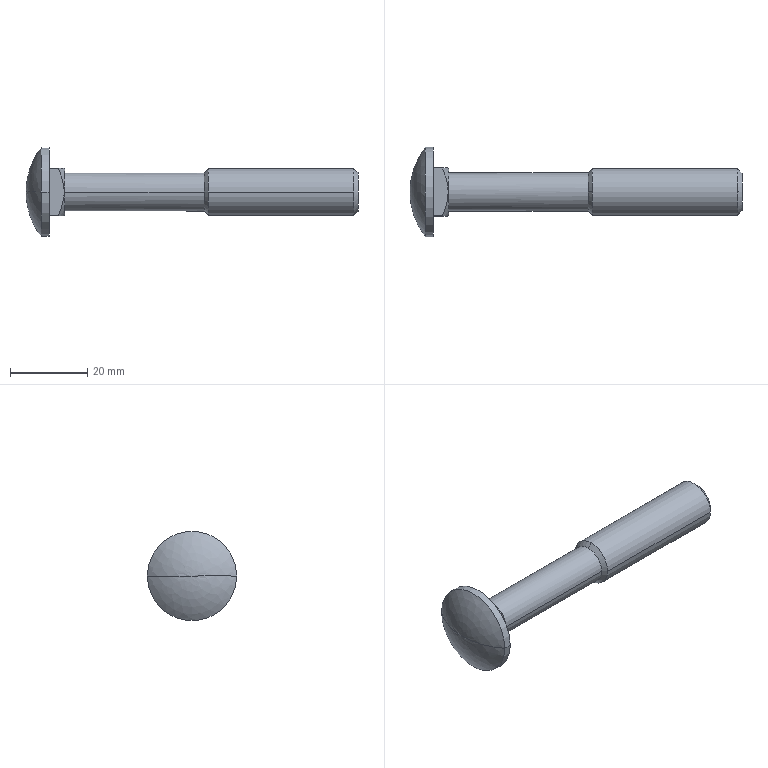Part | SolidWorks | features BaseBody 1 | 1 solid | 21 faces | box 86 x 23.16 x 23.16 mm | volume 9538 mm3 | plane 7 | cylinder 6 | cone 6 | spline 2 | commonest cylinder face diameters 9.853 x2 12 x2 23.16 x2
STEP:
#1=CARTESIAN_POINT('',(-2.,-11.58,0.));
#2=VERTEX_POINT('',#1);
#3=CARTESIAN_POINT('',(-2.,11.58,0.));
#4=VERTEX_POINT('',#3);
#5=CARTESIAN_POINT('',(-2.,0.,0.));
#6=DIRECTION('',(1.,0.,0.));
#7=DIRECTION('',(0.,1.,0.));
#8=AXIS2_PLACEMENT_3D('',#5,#6,#7);
#9=CIRCLE('',#8,11.58);
#10=EDGE_CURVE('',#2,#4,#9,.T.);
#11=ORIENTED_EDGE('',*,*,#10,.F.);
#12=CARTESIAN_POINT('',(-6.,0.,0.));
#13=VERTEX_POINT('',#12);
#14=CARTESIAN_POINT('',(12.762,0.,0.));
#15=DIRECTION('',(0.,0.,-1.));
#16=DIRECTION('',(1.,0.,0.));
#17=AXIS2_PLACEMENT_3D('',#14,#15,#16);
#18=CIRCLE('',#17,18.762);
#19=EDGE_CURVE('',#2,#13,#18,.T.);
#20=ORIENTED_EDGE('',*,*,#19,.T.);
#21=CARTESIAN_POINT('',(12.762,0.,0.));
#22=DIRECTION('',(0.,0.,1.));
#23=DIRECTION('',(1.,0.,0.));
#24=AXIS2_PLACEMENT_3D('',#21,#22,#23);
#25=CIRCLE('',#24,18.762);
#26=EDGE_CURVE('',#4,#13,#25,.T.);
#27=ORIENTED_EDGE('',*,*,#26,.F.);
#28=EDGE_LOOP('',(#11,#20,#27));
#29=FACE_OUTER_BOUND('',#28,.T.);
#30=CARTESIAN_POINT('',(-2.,-11.58,0.));
#31=CARTESIAN_POINT('',(-2.,-11.58,-23.16));
#32=CARTESIAN_POINT('',(-2.,11.58,-23.16));
#33=CARTESIAN_POINT('',(-2.,11.58,0.));
#34=CARTESIAN_POINT('',(-4.616,-8.245,0.));
#35=CARTESIAN_POINT('',(-4.616,-8.245,-16.49));
#36=CARTESIAN_POINT('',(-4.616,8.245,-16.49));
#37=CARTESIAN_POINT('',(-4.616,8.245,0.));
#38=CARTESIAN_POINT('',(-6.,-4.239,0.));
#39=CARTESIAN_POINT('',(-6.,-4.239,-8.477));
#40=CARTESIAN_POINT('',(-6.,4.239,-8.477));
#41=CARTESIAN_POINT('',(-6.,4.239,0.));
#42=CARTESIAN_POINT('',(-6.,0.,0.));
#43=CARTESIAN_POINT('',(-6.,0.,0.));
#44=CARTESIAN_POINT('',(-6.,0.,0.));
#45=CARTESIAN_POINT('',(-6.,0.,0.));
#46=(BOUNDED_SURFACE()B_SPLINE_SURFACE(3,3,((#30,#31,#32,#33),(#34,#35,#36,#37),(#38,#39,#40,#41),(#42,#43,#44,#45)),.UNSPECIFIED.,.F.,.F.,.F.)B_SPLINE_SURFACE_WITH_KNOTS((4,4),(4,4),(0.,1.),(0.,1.),.UNSPECIFIED.)GEOMETRIC_REPRESENTATION_ITEM()RATIONAL_B_SPLINE_SURFACE(((1.,0.3333,0.3333,1.),(0.9635,0.3212,0.3212,0.9635),(0.9635,0.3212,0.3212,0.9635),(1.,0.3333,0.3333,1.)))REPRESENTATION_ITEM('')SURFACE());
#47=ADVANCED_FACE('',(#29),#46,.T.);
#48=CARTESIAN_POINT('',(41.25,0.,6.));
#49=VERTEX_POINT('',#48);
#50=CARTESIAN_POINT('',(41.25,-6.,0.));
#51=VERTEX_POINT('',#50);
#52=CARTESIAN_POINT('',(41.25,0.,0.));
#53=DIRECTION('',(1.,0.,0.));
#54=DIRECTION('',(0.,1.,0.));
#55=AXIS2_PLACEMENT_3D('',#52,#53,#54);
#56=CIRCLE('',#55,6.);
#57=EDGE_CURVE('',#49,#51,#56,.T.);
#58=ORIENTED_EDGE('',*,*,#57,.T.);
#59=CARTESIAN_POINT('',(78.926,-6.,0.));
#60=VERTEX_POINT('',#59);
#61=CARTESIAN_POINT('',(60.625,-6.,0.));
#62=DIRECTION('',(1.,0.,0.));
#63=VECTOR('',#62,1000.);
#64=LINE('',#61,#63);
#65=EDGE_CURVE('',#51,#60,#64,.T.);
#66=ORIENTED_EDGE('',*,*,#65,.T.);
#67=CARTESIAN_POINT('',(78.926,0.,6.));
#68=VERTEX_POINT('',#67);
#69=CARTESIAN_POINT('',(78.926,0.,0.));
#70=DIRECTION('',(-1.,0.,0.));
#71=DIRECTION('',(0.,1.,0.));
#72=AXIS2_PLACEMENT_3D('',#69,#70,#71);
#73=CIRCLE('',#72,6.);
#74=EDGE_CURVE('',#60,#68,#73,.T.);
#75=ORIENTED_EDGE('',*,*,#74,.T.);
#76=CARTESIAN_POINT('',(78.926,6.,0.));
#77=VERTEX_POINT('',#76);
#78=CARTESIAN_POINT('',(78.926,0.,0.));
#79=DIRECTION('',(-1.,0.,0.));
#80=DIRECTION('',(0.,1.,0.));
#81=AXIS2_PLACEMENT_3D('',#78,#79,#80);
#82=CIRCLE('',#81,6.);
#83=EDGE_CURVE('',#68,#77,#82,.T.);
#84=ORIENTED_EDGE('',*,*,#83,.T.);
#85=CARTESIAN_POINT('',(41.25,6.,0.));
#86=VERTEX_POINT('',#85);
#87=CARTESIAN_POINT('',(60.625,6.,0.));
#88=DIRECTION('',(1.,0.,0.));
#89=VECTOR('',#88,1000.);
#90=LINE('',#87,#89);
#91=EDGE_CURVE('',#86,#77,#90,.T.);
#92=ORIENTED_EDGE('',*,*,#91,.F.);
#93=CARTESIAN_POINT('',(41.25,0.,0.));
#94=DIRECTION('',(1.,0.,0.));
#95=DIRECTION('',(0.,1.,0.));
#96=AXIS2_PLACEMENT_3D('',#93,#94,#95);
#97=CIRCLE('',#96,6.);
#98=EDGE_CURVE('',#86,#49,#97,.T.);
#99=ORIENTED_EDGE('',*,*,#98,.T.);
#100=EDGE_LOOP('',(#58,#66,#75,#84,#92,#99));
#101=FACE_OUTER_BOUND('',#100,.T.);
#102=CARTESIAN_POINT('',(60.625,0.,0.));
#103=DIRECTION('',(1.,0.,0.));
#104=DIRECTION('',(0.,1.,0.));
#105=AXIS2_PLACEMENT_3D('',#102,#103,#104);
#106=CYLINDRICAL_SURFACE('',#105,6.);
#107=ADVANCED_FACE('',(#101),#106,.T.);
#108=CARTESIAN_POINT('',(80.,0.,4.926));
#109=VERTEX_POINT('',#108);
#110=CARTESIAN_POINT('',(80.,0.,-4.926));
#111=VERTEX_POINT('',#110);
#112=CARTESIAN_POINT('',(80.,0.,0.));
#113=DIRECTION('',(-1.,0.,0.));
#114=DIRECTION('',(0.,0.,1.));
#115=AXIS2_PLACEMENT_3D('',#112,#113,#114);
#116=CIRCLE('',#115,4.926);
#117=EDGE_CURVE('',#109,#111,#116,.T.);
#118=ORIENTED_EDGE('',*,*,#117,.T.);
#119=CARTESIAN_POINT('',(78.926,0.,-6.));
#120=VERTEX_POINT('',#119);
#121=CARTESIAN_POINT('',(78.926,0.,-6.));
#122=DIRECTION('',(-0.7071,0.,-0.7071));
#123=VECTOR('',#122,1000.);
#124=LINE('',#121,#123);
#125=EDGE_CURVE('',#111,#120,#124,.T.);
#126=ORIENTED_EDGE('',*,*,#125,.T.);
#127=CARTESIAN_POINT('',(78.926,0.,0.));
#128=DIRECTION('',(-1.,0.,0.));
#129=DIRECTION('',(0.,1.,0.));
#130=AXIS2_PLACEMENT_3D('',#127,#128,#129);
#131=CIRCLE('',#130,6.);
#132=EDGE_CURVE('',#77,#120,#131,.T.);
#133=ORIENTED_EDGE('',*,*,#132,.F.);
#134=ORIENTED_EDGE('',*,*,#83,.F.);
#135=CARTESIAN_POINT('',(78.926,0.,6.));
#136=DIRECTION('',(-0.7071,0.,0.7071));
#137=VECTOR('',#136,1000.);
#138=LINE('',#135,#137);
#139=EDGE_CURVE('',#109,#68,#138,.T.);
#140=ORIENTED_EDGE('',*,*,#139,.F.);
#141=EDGE_LOOP('',(#118,#126,#133,#134,#140));
#142=FACE_OUTER_BOUND('',#141,.T.);
#143=CARTESIAN_POINT('',(78.926,0.,0.));
#144=DIRECTION('',(-1.,0.,0.));
#145=DIRECTION('',(0.,0.,1.));
#146=AXIS2_PLACEMENT_3D('',#143,#144,#145);
#147=CONICAL_SURFACE('',#146,6.,0.7854);
#148=ADVANCED_FACE('',(#142),#147,.T.);
#149=CARTESIAN_POINT('',(40.176,4.926,0.));
#150=VERTEX_POINT('',#149);
#151=CARTESIAN_POINT('',(40.176,0.,4.926));
#152=VERTEX_POINT('',#151);
#153=CARTESIAN_POINT('',(40.176,0.,0.));
#154=DIRECTION('',(1.,0.,0.));
#155=DIRECTION('',(0.,1.,0.));
#156=AXIS2_PLACEMENT_3D('',#153,#154,#155);
#157=CIRCLE('',#156,4.926);
#158=EDGE_CURVE('',#150,#152,#157,.T.);
#159=ORIENTED_EDGE('',*,*,#158,.T.);
#160=CARTESIAN_POINT('',(41.25,0.,6.));
#161=DIRECTION('',(0.7071,0.,0.7071));
#162=VECTOR('',#161,1000.);
#163=LINE('',#160,#162);
#164=EDGE_CURVE('',#152,#49,#163,.T.);
#165=ORIENTED_EDGE('',*,*,#164,.T.);
#166=ORIENTED_EDGE('',*,*,#98,.F.);
#167=CARTESIAN_POINT('',(41.25,0.,-6.));
#168=VERTEX_POINT('',#167);
#169=CARTESIAN_POINT('',(41.25,0.,0.));
#170=DIRECTION('',(1.,0.,0.));
#171=DIRECTION('',(0.,1.,0.));
#172=AXIS2_PLACEMENT_3D('',#169,#170,#171);
#173=CIRCLE('',#172,6.);
#174=EDGE_CURVE('',#168,#86,#173,.T.);
#175=ORIENTED_EDGE('',*,*,#174,.F.);
#176=CARTESIAN_POINT('',(40.176,0.,-4.926));
#177=VERTEX_POINT('',#176);
#178=CARTESIAN_POINT('',(41.25,0.,-6.));
#179=DIRECTION('',(0.7071,0.,-0.7071));
#180=VECTOR('',#179,1000.);
#181=LINE('',#178,#180);
#182=EDGE_CURVE('',#177,#168,#181,.T.);
#183=ORIENTED_EDGE('',*,*,#182,.F.);
#184=CARTESIAN_POINT('',(40.176,0.,0.));
#185=DIRECTION('',(1.,0.,0.));
#186=DIRECTION('',(0.,1.,0.));
#187=AXIS2_PLACEMENT_3D('',#184,#185,#186);
#188=CIRCLE('',#187,4.926);
#189=EDGE_CURVE('',#177,#150,#188,.T.);
#190=ORIENTED_EDGE('',*,*,#189,.T.);
#191=EDGE_LOOP('',(#159,#165,#166,#175,#183,#190));
#192=FACE_OUTER_BOUND('',#191,.T.);
#193=CARTESIAN_POINT('',(41.25,0.,0.));
#194=DIRECTION('',(1.,0.,0.));
#195=DIRECTION('',(0.,0.,-1.));
#196=AXIS2_PLACEMENT_3D('',#193,#194,#195);
#197=CONICAL_SURFACE('',#196,6.,0.7854);
#198=ADVANCED_FACE('',(#192),#197,.T.);
#199=CARTESIAN_POINT('',(4.,4.926,0.));
#200=VERTEX_POINT('',#199);
#201=CARTESIAN_POINT('',(4.,-4.926,0.));
#202=VERTEX_POINT('',#201);
#203=CARTESIAN_POINT('',(4.,0.,0.));
#204=DIRECTION('',(1.,0.,0.));
#205=DIRECTION('',(0.,1.,0.));
#206=AXIS2_PLACEMENT_3D('',#203,#204,#205);
#207=CIRCLE('',#206,4.926);
#208=EDGE_CURVE('',#200,#202,#207,.T.);
#209=ORIENTED_EDGE('',*,*,#208,.T.);
#210=CARTESIAN_POINT('',(40.176,-4.926,0.));
#211=VERTEX_POINT('',#210);
#212=CARTESIAN_POINT('',(22.088,-4.926,0.));
#213=DIRECTION('',(1.,0.,0.));
#214=VECTOR('',#213,1000.);
#215=LINE('',#212,#214);
#216=EDGE_CURVE('',#202,#211,#215,.T.);
#217=ORIENTED_EDGE('',*,*,#216,.T.);
#218=CARTESIAN_POINT('',(40.176,0.,0.));
#219=DIRECTION('',(1.,0.,0.));
#220=DIRECTION('',(0.,1.,0.));
#221=AXIS2_PLACEMENT_3D('',#218,#219,#220);
#222=CIRCLE('',#221,4.926);
#223=EDGE_CURVE('',#152,#211,#222,.T.);
#224=ORIENTED_EDGE('',*,*,#223,.F.);
#225=ORIENTED_EDGE('',*,*,#158,.F.);
#226=CARTESIAN_POINT('',(22.088,4.926,0.));
#227=DIRECTION('',(1.,0.,0.));
#228=VECTOR('',#227,1000.);
#229=LINE('',#226,#228);
#230=EDGE_CURVE('',#200,#150,#229,.T.);
#231=ORIENTED_EDGE('',*,*,#230,.F.);
#232=EDGE_LOOP('',(#209,#217,#224,#225,#231));
#233=FACE_OUTER_BOUND('',#232,.T.);
#234=CARTESIAN_POINT('',(22.088,0.,0.));
#235=DIRECTION('',(1.,0.,0.));
#236=DIRECTION('',(0.,1.,0.));
#237=AXIS2_PLACEMENT_3D('',#234,#235,#236);
#238=CYLINDRICAL_SURFACE('',#237,4.926);
#239=ADVANCED_FACE('',(#233),#238,.T.);
#240=CARTESIAN_POINT('',(4.,0.,-6.));
#241=VERTEX_POINT('',#240);
#242=CARTESIAN_POINT('',(4.,0.,6.));
#243=VERTEX_POINT('',#242);
#244=CARTESIAN_POINT('',(4.,0.,0.));
#245=DIRECTION('',(1.,0.,0.));
#246=DIRECTION('',(0.,0.,1.));
#247=AXIS2_PLACEMENT_3D('',#244,#245,#246);
#248=CIRCLE('',#247,6.);
#249=EDGE_CURVE('',#241,#243,#248,.T.);
#250=ORIENTED_EDGE('',*,*,#249,.F.);
#251=CARTESIAN_POINT('',(3.876,0.,-6.215));
#252=VERTEX_POINT('',#251);
#253=CARTESIAN_POINT('',(2.38,0.,-8.806));
#254=DIRECTION('',(-0.5,0.,-0.866));
#255=VECTOR('',#254,1000.);
#256=LINE('',#253,#255);
#257=EDGE_CURVE('',#241,#252,#256,.T.);
#258=ORIENTED_EDGE('',*,*,#257,.T.);
#259=CARTESIAN_POINT('',(2.39,6.215,-6.215));
#260=VERTEX_POINT('',#259);
#261=CARTESIAN_POINT('',(3.876,0.,-6.215));
#262=CARTESIAN_POINT('',(3.876,1.07,-6.215));
#263=CARTESIAN_POINT('',(3.711,2.121,-6.215));
#264=CARTESIAN_POINT('',(3.302,3.681,-6.215));
#265=CARTESIAN_POINT('',(3.141,4.197,-6.215));
#266=CARTESIAN_POINT('',(2.786,5.213,-6.215));
#267=CARTESIAN_POINT('',(2.593,5.716,-6.215));
#268=CARTESIAN_POINT('',(2.39,6.215,-6.215));
#269=B_SPLINE_CURVE_WITH_KNOTS('',3,(#261,#262,#263,#264,#265,#266,#267,#268),.UNSPECIFIED.,.F.,.F.,(4,2,2,4),(0.006403,0.009604,0.0112,0.01281),.UNSPECIFIED.);
#270=EDGE_CURVE('',#252,#260,#269,.T.);
#271=ORIENTED_EDGE('',*,*,#270,.T.);
#272=CARTESIAN_POINT('',(2.39,6.215,6.215));
#273=VERTEX_POINT('',#272);
#274=CARTESIAN_POINT('',(2.39,6.215,-6.215));
#275=CARTESIAN_POINT('',(2.796,6.215,-5.22));
#276=CARTESIAN_POINT('',(3.161,6.215,-4.214));
#277=CARTESIAN_POINT('',(3.569,6.215,-2.666));
#278=CARTESIAN_POINT('',(3.68,6.215,-2.143));
#279=CARTESIAN_POINT('',(3.834,6.215,-1.079));
#280=CARTESIAN_POINT('',(3.876,6.215,-0.535));
#281=CARTESIAN_POINT('',(3.876,6.215,1.07));
#282=CARTESIAN_POINT('',(3.711,6.215,2.121));
#283=CARTESIAN_POINT('',(3.302,6.215,3.681));
#284=CARTESIAN_POINT('',(3.141,6.215,4.197));
#285=CARTESIAN_POINT('',(2.786,6.215,5.213));
#286=CARTESIAN_POINT('',(2.593,6.215,5.716));
#287=CARTESIAN_POINT('',(2.39,6.215,6.215));
#288=B_SPLINE_CURVE_WITH_KNOTS('',3,(#274,#275,#276,#277,#278,#279,#280,#281,#282,#283,#284,#285,#286,#287),.UNSPECIFIED.,.F.,.F.,(4,2,2,2,2,2,4),(0.,0.003201,0.004802,0.006403,0.009604,0.0112,0.01281),.UNSPECIFIED.);
#289=EDGE_CURVE('',#260,#273,#288,.T.);
#290=ORIENTED_EDGE('',*,*,#289,.T.);
#291=CARTESIAN_POINT('',(3.876,0.,6.215));
#292=VERTEX_POINT('',#291);
#293=CARTESIAN_POINT('',(2.39,6.215,6.215));
#294=CARTESIAN_POINT('',(2.796,5.22,6.215));
#295=CARTESIAN_POINT('',(3.161,4.214,6.215));
#296=CARTESIAN_POINT('',(3.569,2.666,6.215));
#297=CARTESIAN_POINT('',(3.68,2.143,6.215));
#298=CARTESIAN_POINT('',(3.834,1.079,6.215));
#299=CARTESIAN_POINT('',(3.876,0.5349,6.215));
#300=CARTESIAN_POINT('',(3.876,0.,6.215));
#301=B_SPLINE_CURVE_WITH_KNOTS('',3,(#293,#294,#295,#296,#297,#298,#299,#300),.UNSPECIFIED.,.F.,.F.,(4,2,2,4),(0.,0.003201,0.004802,0.006403),.UNSPECIFIED.);
#302=EDGE_CURVE('',#273,#292,#301,.T.);
#303=ORIENTED_EDGE('',*,*,#302,.T.);
#304=CARTESIAN_POINT('',(2.38,0.,8.806));
#305=DIRECTION('',(-0.5,0.,0.866));
#306=VECTOR('',#305,1000.);
#307=LINE('',#304,#306);
#308=EDGE_CURVE('',#243,#292,#307,.T.);
#309=ORIENTED_EDGE('',*,*,#308,.F.);
#310=EDGE_LOOP('',(#250,#258,#271,#290,#303,#309));
#311=FACE_OUTER_BOUND('',#310,.T.);
#312=CARTESIAN_POINT('',(2.38,0.,0.));
#313=DIRECTION('',(-1.,0.,0.));
#314=DIRECTION('',(0.,0.,1.));
#315=AXIS2_PLACEMENT_3D('',#312,#313,#314);
#316=CONICAL_SURFACE('',#315,8.806,1.047);
#317=ADVANCED_FACE('',(#311),#316,.T.);
#318=CARTESIAN_POINT('',(-2.,0.,0.));
#319=DIRECTION('',(1.,0.,0.));
#320=DIRECTION('',(0.,1.,0.));
#321=AXIS2_PLACEMENT_3D('',#318,#319,#320);
#322=CIRCLE('',#321,11.58);
#323=EDGE_CURVE('',#4,#2,#322,.T.);
#324=ORIENTED_EDGE('',*,*,#323,.T.);
#325=CARTESIAN_POINT('',(0.,-11.58,0.));
#326=VERTEX_POINT('',#325);
#327=CARTESIAN_POINT('',(-1.,-11.58,0.));
#328=DIRECTION('',(1.,0.,0.));
#329=VECTOR('',#328,1000.);
#330=LINE('',#327,#329);
#331=EDGE_CURVE('',#2,#326,#330,.T.);
#332=ORIENTED_EDGE('',*,*,#331,.T.);
#333=CARTESIAN_POINT('',(0.,11.58,0.));
#334=VERTEX_POINT('',#333);
#335=CARTESIAN_POINT('',(0.,0.,0.));
#336=DIRECTION('',(1.,0.,0.));
#337=DIRECTION('',(0.,1.,0.));
#338=AXIS2_PLACEMENT_3D('',#335,#336,#337);
#339=CIRCLE('',#338,11.58);
#340=EDGE_CURVE('',#334,#326,#339,.T.);
#341=ORIENTED_EDGE('',*,*,#340,.F.);
#342=CARTESIAN_POINT('',(-1.,11.58,0.));
#343=DIRECTION('',(1.,0.,0.));
#344=VECTOR('',#343,1000.);
#345=LINE('',#342,#344);
#346=EDGE_CURVE('',#4,#334,#345,.T.);
#347=ORIENTED_EDGE('',*,*,#346,.F.);
#348=EDGE_LOOP('',(#324,#332,#341,#347));
#349=FACE_OUTER_BOUND('',#348,.T.);
#350=CARTESIAN_POINT('',(-1.,0.,0.));
#351=DIRECTION('',(1.,0.,0.));
#352=DIRECTION('',(0.,1.,0.));
#353=AXIS2_PLACEMENT_3D('',#350,#351,#352);
#354=CYLINDRICAL_SURFACE('',#353,11.58);
#355=ADVANCED_FACE('',(#349),#354,.T.);
#356=ORIENTED_EDGE('',*,*,#65,.F.);
#357=CARTESIAN_POINT('',(41.25,0.,0.));
#358=DIRECTION('',(1.,0.,0.));
#359=DIRECTION('',(0.,1.,0.));
#360=AXIS2_PLACEMENT_3D('',#357,#358,#359);
#361=CIRCLE('',#360,6.);
#362=EDGE_CURVE('',#51,#168,#361,.T.);
#363=ORIENTED_EDGE('',*,*,#362,.T.);
#364=ORIENTED_EDGE('',*,*,#174,.T.);
#365=ORIENTED_EDGE('',*,*,#91,.T.);
#366=ORIENTED_EDGE('',*,*,#132,.T.);
#367=CARTESIAN_POINT('',(78.926,0.,0.));
#368=DIRECTION('',(-1.,0.,0.));
#369=DIRECTION('',(0.,1.,0.));
#370=AXIS2_PLACEMENT_3D('',#367,#368,#369);
#371=CIRCLE('',#370,6.);
#372=EDGE_CURVE('',#120,#60,#371,.T.);
#373=ORIENTED_EDGE('',*,*,#372,.T.);
#374=EDGE_LOOP('',(#356,#363,#364,#365,#366,#373));
#375=FACE_OUTER_BOUND('',#374,.T.);
#376=CARTESIAN_POINT('',(60.625,0.,0.));
#377=DIRECTION('',(1.,0.,0.));
#378=DIRECTION('',(0.,1.,0.));
#379=AXIS2_PLACEMENT_3D('',#376,#377,#378);
#380=CYLINDRICAL_SURFACE('',#379,6.);
#381=ADVANCED_FACE('',(#375),#380,.T.);
#382=ORIENTED_EDGE('',*,*,#125,.F.);
#383=CARTESIAN_POINT('',(80.,0.,0.));
#384=DIRECTION('',(-1.,0.,0.));
#385=DIRECTION('',(0.,0.,1.));
#386=AXIS2_PLACEMENT_3D('',#383,#384,#385);
#387=CIRCLE('',#386,4.926);
#388=EDGE_CURVE('',#111,#109,#387,.T.);
#389=ORIENTED_EDGE('',*,*,#388,.T.);
#390=ORIENTED_EDGE('',*,*,#139,.T.);
#391=ORIENTED_EDGE('',*,*,#74,.F.);
#392=ORIENTED_EDGE('',*,*,#372,.F.);
#393=EDGE_LOOP('',(#382,#389,#390,#391,#392));
#394=FACE_OUTER_BOUND('',#393,.T.);
#395=CARTESIAN_POINT('',(78.926,0.,0.));
#396=DIRECTION('',(-1.,0.,0.));
#397=DIRECTION('',(0.,0.,1.));
#398=AXIS2_PLACEMENT_3D('',#395,#396,#397);
#399=CONICAL_SURFACE('',#398,6.,0.7854);
#400=ADVANCED_FACE('',(#394),#399,.T.);
#401=ORIENTED_EDGE('',*,*,#164,.F.);
#402=ORIENTED_EDGE('',*,*,#223,.T.);
#403=CARTESIAN_POINT('',(40.176,0.,0.));
#404=DIRECTION('',(1.,0.,0.));
#405=DIRECTION('',(0.,1.,0.));
#406=AXIS2_PLACEMENT_3D('',#403,#404,#405);
#407=CIRCLE('',#406,4.926);
#408=EDGE_CURVE('',#211,#177,#407,.T.);
#409=ORIENTED_EDGE('',*,*,#408,.T.);
#410=ORIENTED_EDGE('',*,*,#182,.T.);
#411=ORIENTED_EDGE('',*,*,#362,.F.);
#412=ORIENTED_EDGE('',*,*,#57,.F.);
#413=EDGE_LOOP('',(#401,#402,#409,#410,#411,#412));
#414=FACE_OUTER_BOUND('',#413,.T.);
#415=CARTESIAN_POINT('',(41.25,0.,0.));
#416=DIRECTION('',(1.,0.,0.));
#417=DIRECTION('',(0.,0.,-1.));
#418=AXIS2_PLACEMENT_3D('',#415,#416,#417);
#419=CONICAL_SURFACE('',#418,6.,0.7854);
#420=ADVANCED_FACE('',(#414),#419,.T.);
#421=ORIENTED_EDGE('',*,*,#117,.F.);
#422=ORIENTED_EDGE('',*,*,#388,.F.);
#423=EDGE_LOOP('',(#421,#422));
#424=FACE_OUTER_BOUND('',#423,.T.);
#425=CARTESIAN_POINT('',(80.,3.,0.));
#426=DIRECTION('',(1.,0.,0.));
#427=DIRECTION('',(0.,1.,0.));
#428=AXIS2_PLACEMENT_3D('',#425,#426,#427);
#429=PLANE('',#428);
#430=ADVANCED_FACE('',(#424),#429,.T.);
#431=ORIENTED_EDGE('',*,*,#216,.F.);
#432=CARTESIAN_POINT('',(4.,0.,0.));
#433=DIRECTION('',(1.,0.,0.));
#434=DIRECTION('',(0.,1.,0.));
#435=AXIS2_PLACEMENT_3D('',#432,#433,#434);
#436=CIRCLE('',#435,4.926);
#437=EDGE_CURVE('',#202,#200,#436,.T.);
#438=ORIENTED_EDGE('',*,*,#437,.T.);
#439=ORIENTED_EDGE('',*,*,#230,.T.);
#440=ORIENTED_EDGE('',*,*,#189,.F.);
#441=ORIENTED_EDGE('',*,*,#408,.F.);
#442=EDGE_LOOP('',(#431,#438,#439,#440,#441));
#443=FACE_OUTER_BOUND('',#442,.T.);
#444=CARTESIAN_POINT('',(22.088,0.,0.));
#445=DIRECTION('',(1.,0.,0.));
#446=DIRECTION('',(0.,1.,0.));
#447=AXIS2_PLACEMENT_3D('',#444,#445,#446);
#448=CYLINDRICAL_SURFACE('',#447,4.926);
#449=ADVANCED_FACE('',(#443),#448,.T.);
#450=ORIENTED_EDGE('',*,*,#208,.F.);
#451=ORIENTED_EDGE('',*,*,#437,.F.);
#452=EDGE_LOOP('',(#450,#451));
#453=FACE_BOUND('',#452,.T.);
#454=CARTESIAN_POINT('',(4.,0.,0.));
#455=DIRECTION('',(1.,0.,0.));
#456=DIRECTION('',(0.,0.,1.));
#457=AXIS2_PLACEMENT_3D('',#454,#455,#456);
#458=CIRCLE('',#457,6.);
#459=EDGE_CURVE('',#243,#241,#458,.T.);
#460=ORIENTED_EDGE('',*,*,#459,.T.);
#461=ORIENTED_EDGE('',*,*,#249,.T.);
#462=EDGE_LOOP('',(#460,#461));
#463=FACE_OUTER_BOUND('',#462,.T.);
#464=CARTESIAN_POINT('',(4.,0.,0.));
#465=DIRECTION('',(1.,0.,0.));
#466=DIRECTION('',(0.,0.,-1.));
#467=AXIS2_PLACEMENT_3D('',#464,#465,#466);
#468=PLANE('',#467);
#469=ADVANCED_FACE('',(#453,#463),#468,.T.);
#470=ORIENTED_EDGE('',*,*,#257,.F.);
#471=ORIENTED_EDGE('',*,*,#459,.F.);
#472=ORIENTED_EDGE('',*,*,#308,.T.);
#473=CARTESIAN_POINT('',(2.39,-6.215,6.215));
#474=VERTEX_POINT('',#473);
#475=CARTESIAN_POINT('',(3.876,0.,6.215));
#476=CARTESIAN_POINT('',(3.876,-1.07,6.215));
#477=CARTESIAN_POINT('',(3.711,-2.121,6.215));
#478=CARTESIAN_POINT('',(3.302,-3.681,6.215));
#479=CARTESIAN_POINT('',(3.141,-4.197,6.215));
#480=CARTESIAN_POINT('',(2.786,-5.213,6.215));
#481=CARTESIAN_POINT('',(2.593,-5.716,6.215));
#482=CARTESIAN_POINT('',(2.39,-6.215,6.215));
#483=B_SPLINE_CURVE_WITH_KNOTS('',3,(#475,#476,#477,#478,#479,#480,#481,#482),.UNSPECIFIED.,.F.,.F.,(4,2,2,4),(0.006403,0.009604,0.0112,0.01281),.UNSPECIFIED.);
#484=EDGE_CURVE('',#292,#474,#483,.T.);
#485=ORIENTED_EDGE('',*,*,#484,.T.);
#486=CARTESIAN_POINT('',(2.39,-6.215,-6.215));
#487=VERTEX_POINT('',#486);
#488=CARTESIAN_POINT('',(2.39,-6.215,6.215));
#489=CARTESIAN_POINT('',(2.796,-6.215,5.22));
#490=CARTESIAN_POINT('',(3.161,-6.215,4.214));
#491=CARTESIAN_POINT('',(3.569,-6.215,2.666));
#492=CARTESIAN_POINT('',(3.68,-6.215,2.143));
#493=CARTESIAN_POINT('',(3.834,-6.215,1.079));
#494=CARTESIAN_POINT('',(3.876,-6.215,0.535));
#495=CARTESIAN_POINT('',(3.876,-6.215,-1.07));
#496=CARTESIAN_POINT('',(3.711,-6.215,-2.121));
#497=CARTESIAN_POINT('',(3.302,-6.215,-3.681));
#498=CARTESIAN_POINT('',(3.141,-6.215,-4.197));
#499=CARTESIAN_POINT('',(2.786,-6.215,-5.213));
#500=CARTESIAN_POINT('',(2.593,-6.215,-5.716));
#501=CARTESIAN_POINT('',(2.39,-6.215,-6.215));
#502=B_SPLINE_CURVE_WITH_KNOTS('',3,(#488,#489,#490,#491,#492,#493,#494,#495,#496,#497,#498,#499,#500,#501),.UNSPECIFIED.,.F.,.F.,(4,2,2,2,2,2,4),(0.,0.003201,0.004802,0.006403,0.009604,0.0112,0.01281),.UNSPECIFIED.);
#503=EDGE_CURVE('',#474,#487,#502,.T.);
#504=ORIENTED_EDGE('',*,*,#503,.T.);
#505=CARTESIAN_POINT('',(2.39,-6.215,-6.215));
#506=CARTESIAN_POINT('',(2.796,-5.22,-6.215));
#507=CARTESIAN_POINT('',(3.161,-4.214,-6.215));
#508=CARTESIAN_POINT('',(3.569,-2.666,-6.215));
#509=CARTESIAN_POINT('',(3.68,-2.143,-6.215));
#510=CARTESIAN_POINT('',(3.834,-1.079,-6.215));
#511=CARTESIAN_POINT('',(3.876,-0.5349,-6.215));
#512=CARTESIAN_POINT('',(3.876,0.,-6.215));
#513=B_SPLINE_CURVE_WITH_KNOTS('',3,(#505,#506,#507,#508,#509,#510,#511,#512),.UNSPECIFIED.,.F.,.F.,(4,2,2,4),(0.,0.003201,0.004802,0.006403),.UNSPECIFIED.);
#514=EDGE_CURVE('',#487,#252,#513,.T.);
#515=ORIENTED_EDGE('',*,*,#514,.T.);
#516=EDGE_LOOP('',(#470,#471,#472,#485,#504,#515));
#517=FACE_OUTER_BOUND('',#516,.T.);
#518=CARTESIAN_POINT('',(2.38,0.,0.));
#519=DIRECTION('',(-1.,0.,0.));
#520=DIRECTION('',(0.,0.,1.));
#521=AXIS2_PLACEMENT_3D('',#518,#519,#520);
#522=CONICAL_SURFACE('',#521,8.806,1.047);
#523=ADVANCED_FACE('',(#517),#522,.T.);
#524=CARTESIAN_POINT('',(0.,6.215,-6.215));
#525=VERTEX_POINT('',#524);
#526=CARTESIAN_POINT('',(0.,6.215,6.215));
#527=VERTEX_POINT('',#526);
#528=CARTESIAN_POINT('',(0.,6.215,0.));
#529=DIRECTION('',(0.,0.,1.));
#530=VECTOR('',#529,1000.);
#531=LINE('',#528,#530);
#532=EDGE_CURVE('',#525,#527,#531,.T.);
#533=ORIENTED_EDGE('',*,*,#532,.T.);
#534=CARTESIAN_POINT('',(0.,6.215,6.215));
#535=DIRECTION('',(1.,0.,0.));
#536=VECTOR('',#535,1000.);
#537=LINE('',#534,#536);
#538=EDGE_CURVE('',#527,#273,#537,.T.);
#539=ORIENTED_EDGE('',*,*,#538,.T.);
#540=ORIENTED_EDGE('',*,*,#289,.F.);
#541=CARTESIAN_POINT('',(0.,6.215,-6.215));
#542=DIRECTION('',(-1.,0.,0.));
#543=VECTOR('',#542,1000.);
#544=LINE('',#541,#543);
#545=EDGE_CURVE('',#260,#525,#544,.T.);
#546=ORIENTED_EDGE('',*,*,#545,.T.);
#547=EDGE_LOOP('',(#533,#539,#540,#546));
#548=FACE_OUTER_BOUND('',#547,.T.);
#549=CARTESIAN_POINT('',(0.,6.215,0.));
#550=DIRECTION('',(0.,1.,0.));
#551=DIRECTION('',(0.,0.,1.));
#552=AXIS2_PLACEMENT_3D('',#549,#550,#551);
#553=PLANE('',#552);
#554=ADVANCED_FACE('',(#548),#553,.T.);
#555=CARTESIAN_POINT('',(0.,-6.215,-6.215));
#556=VERTEX_POINT('',#555);
#557=CARTESIAN_POINT('',(0.,0.,-6.215));
#558=DIRECTION('',(0.,1.,0.));
#559=VECTOR('',#558,1000.);
#560=LINE('',#557,#559);
#561=EDGE_CURVE('',#556,#525,#560,.T.);
#562=ORIENTED_EDGE('',*,*,#561,.T.);
#563=ORIENTED_EDGE('',*,*,#545,.F.);
#564=ORIENTED_EDGE('',*,*,#270,.F.);
#565=ORIENTED_EDGE('',*,*,#514,.F.);
#566=CARTESIAN_POINT('',(0.,-6.215,-6.215));
#567=DIRECTION('',(-1.,0.,0.));
#568=VECTOR('',#567,1000.);
#569=LINE('',#566,#568);
#570=EDGE_CURVE('',#487,#556,#569,.T.);
#571=ORIENTED_EDGE('',*,*,#570,.T.);
#572=EDGE_LOOP('',(#562,#563,#564,#565,#571));
#573=FACE_OUTER_BOUND('',#572,.T.);
#574=CARTESIAN_POINT('',(0.,0.,-6.215));
#575=DIRECTION('',(0.,0.,-1.));
#576=DIRECTION('',(0.,1.,0.));
#577=AXIS2_PLACEMENT_3D('',#574,#575,#576);
#578=PLANE('',#577);
#579=ADVANCED_FACE('',(#573),#578,.T.);
#580=CARTESIAN_POINT('',(0.,-6.215,6.215));
#581=VERTEX_POINT('',#580);
#582=CARTESIAN_POINT('',(0.,-6.215,0.));
#583=DIRECTION('',(0.,0.,-1.));
#584=VECTOR('',#583,1000.);
#585=LINE('',#582,#584);
#586=EDGE_CURVE('',#581,#556,#585,.T.);
#587=ORIENTED_EDGE('',*,*,#586,.T.);
#588=ORIENTED_EDGE('',*,*,#570,.F.);
#589=ORIENTED_EDGE('',*,*,#503,.F.);
#590=CARTESIAN_POINT('',(0.,-6.215,6.215));
#591=DIRECTION('',(-1.,0.,0.));
#592=VECTOR('',#591,1000.);
#593=LINE('',#590,#592);
#594=EDGE_CURVE('',#474,#581,#593,.T.);
#595=ORIENTED_EDGE('',*,*,#594,.T.);
#596=EDGE_LOOP('',(#587,#588,#589,#595));
#597=FACE_OUTER_BOUND('',#596,.T.);
#598=CARTESIAN_POINT('',(0.,-6.215,0.));
#599=DIRECTION('',(0.,-1.,0.));
#600=DIRECTION('',(0.,0.,-1.));
#601=AXIS2_PLACEMENT_3D('',#598,#599,#600);
#602=PLANE('',#601);
#603=ADVANCED_FACE('',(#597),#602,.T.);
#604=CARTESIAN_POINT('',(0.,0.,6.215));
#605=DIRECTION('',(0.,-1.,0.));
#606=VECTOR('',#605,1000.);
#607=LINE('',#604,#606);
#608=EDGE_CURVE('',#527,#581,#607,.T.);
#609=ORIENTED_EDGE('',*,*,#608,.T.);
#610=ORIENTED_EDGE('',*,*,#594,.F.);
#611=ORIENTED_EDGE('',*,*,#484,.F.);
#612=ORIENTED_EDGE('',*,*,#302,.F.);
#613=ORIENTED_EDGE('',*,*,#538,.F.);
#614=EDGE_LOOP('',(#609,#610,#611,#612,#613));
#615=FACE_OUTER_BOUND('',#614,.T.);
#616=CARTESIAN_POINT('',(0.,0.,6.215));
#617=DIRECTION('',(0.,0.,1.));
#618=DIRECTION('',(0.,-1.,0.));
#619=AXIS2_PLACEMENT_3D('',#616,#617,#618);
#620=PLANE('',#619);
#621=ADVANCED_FACE('',(#615),#620,.T.);
#622=ORIENTED_EDGE('',*,*,#586,.F.);
#623=ORIENTED_EDGE('',*,*,#608,.F.);
#624=ORIENTED_EDGE('',*,*,#532,.F.);
#625=ORIENTED_EDGE('',*,*,#561,.F.);
#626=EDGE_LOOP('',(#622,#623,#624,#625));
#627=FACE_BOUND('',#626,.T.);
#628=ORIENTED_EDGE('',*,*,#340,.T.);
#629=CARTESIAN_POINT('',(0.,0.,0.));
#630=DIRECTION('',(1.,0.,0.));
#631=DIRECTION('',(0.,1.,0.));
#632=AXIS2_PLACEMENT_3D('',#629,#630,#631);
#633=CIRCLE('',#632,11.58);
#634=EDGE_CURVE('',#326,#334,#633,.T.);
#635=ORIENTED_EDGE('',*,*,#634,.T.);
#636=EDGE_LOOP('',(#628,#635));
#637=FACE_OUTER_BOUND('',#636,.T.);
#638=CARTESIAN_POINT('',(0.,8.253,0.));
#639=DIRECTION('',(1.,0.,0.));
#640=DIRECTION('',(0.,1.,0.));
#641=AXIS2_PLACEMENT_3D('',#638,#639,#640);
#642=PLANE('',#641);
#643=ADVANCED_FACE('',(#627,#637),#642,.T.);
#644=ORIENTED_EDGE('',*,*,#331,.F.);
#645=ORIENTED_EDGE('',*,*,#10,.T.);
#646=ORIENTED_EDGE('',*,*,#346,.T.);
#647=ORIENTED_EDGE('',*,*,#634,.F.);
#648=EDGE_LOOP('',(#644,#645,#646,#647));
#649=FACE_OUTER_BOUND('',#648,.T.);
#650=CARTESIAN_POINT('',(-1.,0.,0.));
#651=DIRECTION('',(1.,0.,0.));
#652=DIRECTION('',(0.,1.,0.));
#653=AXIS2_PLACEMENT_3D('',#650,#651,#652);
#654=CYLINDRICAL_SURFACE('',#653,11.58);
#655=ADVANCED_FACE('',(#649),#654,.T.);
#656=ORIENTED_EDGE('',*,*,#19,.F.);
#657=ORIENTED_EDGE('',*,*,#323,.F.);
#658=ORIENTED_EDGE('',*,*,#26,.T.);
#659=EDGE_LOOP('',(#656,#657,#658));
#660=FACE_OUTER_BOUND('',#659,.T.);
#661=CARTESIAN_POINT('',(-2.,11.58,0.));
#662=CARTESIAN_POINT('',(-2.,11.58,23.16));
#663=CARTESIAN_POINT('',(-2.,-11.58,23.16));
#664=CARTESIAN_POINT('',(-2.,-11.58,0.));
#665=CARTESIAN_POINT('',(-4.616,8.245,0.));
#666=CARTESIAN_POINT('',(-4.616,8.245,16.49));
#667=CARTESIAN_POINT('',(-4.616,-8.245,16.49));
#668=CARTESIAN_POINT('',(-4.616,-8.245,0.));
#669=CARTESIAN_POINT('',(-6.,4.239,0.));
#670=CARTESIAN_POINT('',(-6.,4.239,8.477));
#671=CARTESIAN_POINT('',(-6.,-4.239,8.477));
#672=CARTESIAN_POINT('',(-6.,-4.239,0.));
#673=CARTESIAN_POINT('',(-6.,0.,0.));
#674=CARTESIAN_POINT('',(-6.,0.,0.));
#675=CARTESIAN_POINT('',(-6.,0.,0.));
#676=CARTESIAN_POINT('',(-6.,0.,0.));
#677=(BOUNDED_SURFACE()B_SPLINE_SURFACE(3,3,((#661,#662,#663,#664),(#665,#666,#667,#668),(#669,#670,#671,#672),(#673,#674,#675,#676)),.UNSPECIFIED.,.F.,.F.,.T.)B_SPLINE_SURFACE_WITH_KNOTS((4,4),(4,4),(0.,1.),(0.,1.),.UNSPECIFIED.)GEOMETRIC_REPRESENTATION_ITEM()RATIONAL_B_SPLINE_SURFACE(((1.,0.3333,0.3333,1.),(0.9635,0.3212,0.3212,0.9635),(0.9635,0.3212,0.3212,0.9635),(1.,0.3333,0.3333,1.)))REPRESENTATION_ITEM('')SURFACE());
#678=ADVANCED_FACE('',(#660),#677,.T.);
#679=CLOSED_SHELL('',(#47,#107,#148,#198,#239,#317,#355,#381,#400,#420,#430,#449,#469,#523,#554,#579,#603,#621,#643,#655,#678));
#680=MANIFOLD_SOLID_BREP('',#679);
#681=CARTESIAN_POINT('',(0.,0.,0.));
#682=DIRECTION('',(0.,0.,1.));
#683=DIRECTION('',(1.,0.,0.));
#684=AXIS2_PLACEMENT_3D('',#681,#682,#683);
#685=(LENGTH_UNIT()NAMED_UNIT(*)SI_UNIT(.MILLI.,.METRE.));
#686=UNCERTAINTY_MEASURE_WITH_UNIT(LENGTH_MEASURE(0.00001),#685,'','');
#687=(NAMED_UNIT(*)PLANE_ANGLE_UNIT()SI_UNIT($,.RADIAN.));
#688=(NAMED_UNIT(*)SI_UNIT($,.STERADIAN.)SOLID_ANGLE_UNIT());
#689=(GEOMETRIC_REPRESENTATION_CONTEXT(3)GLOBAL_UNCERTAINTY_ASSIGNED_CONTEXT((#686))GLOBAL_UNIT_ASSIGNED_CONTEXT((#685,#687,#688))REPRESENTATION_CONTEXT('',''));
#690=ADVANCED_BREP_SHAPE_REPRESENTATION('',(#680,#684),#689);